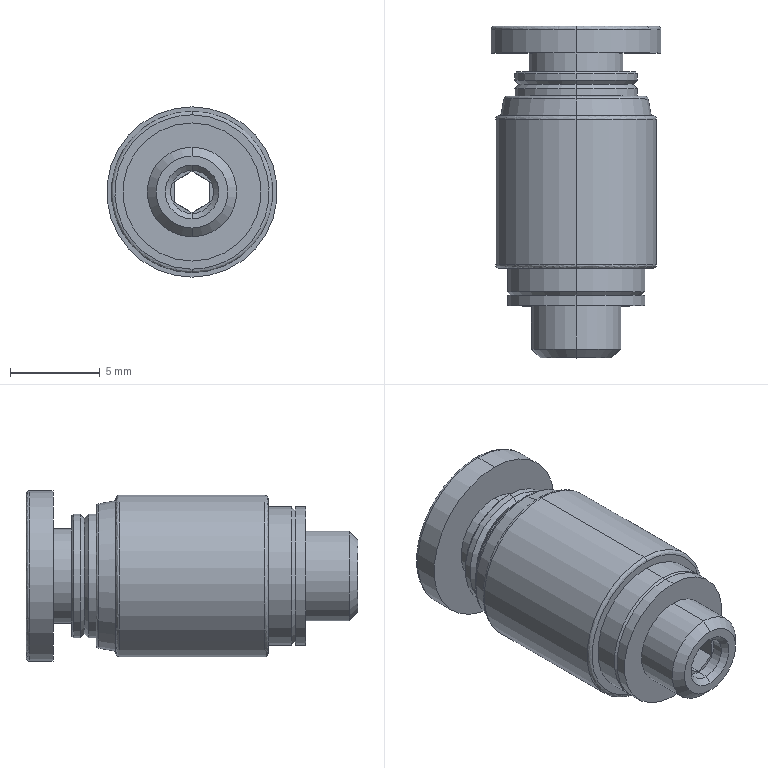Part | STEP file | BPOC4M5 | 1 solid | 62 faces | box 9.5 x 18.5 x 9.5 mm | volume 733.541 mm3 | cylinder 20 | cone 16 | plane 16 | spline 10 | commonest cylinder face diameters 6.9 x4 7.7 x4 2.4 x2 4 x2 5 x2 5.26 x2